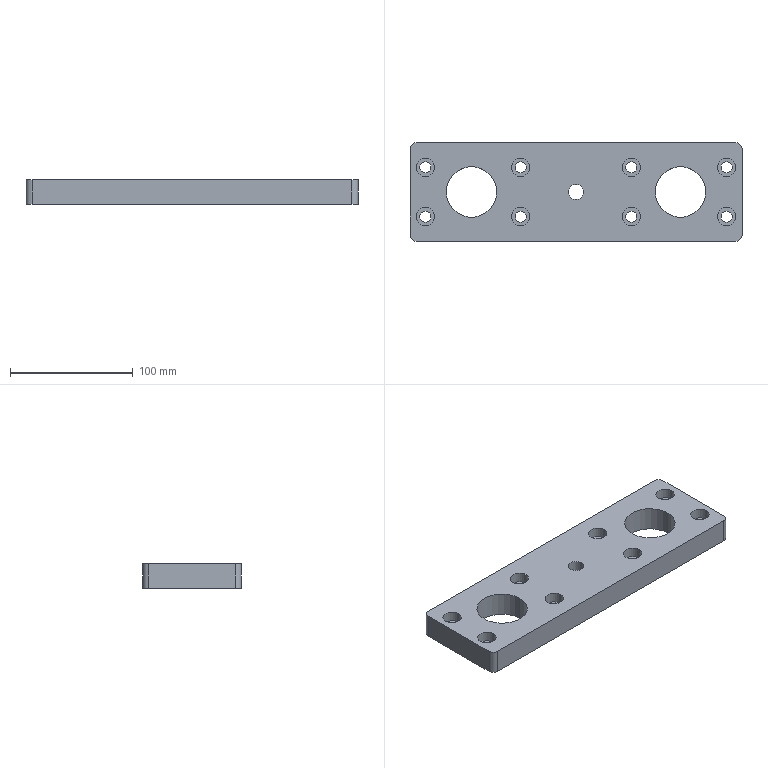Part | STEP file | PN_0006 | 1 solid | 56 faces | box 270 x 80 x 20 mm | volume 358346 mm3 | cylinder 42 | plane 14 | commonest cylinder face diameters 9 x16 15 x16 10 x4 41 x4 12.5 x2